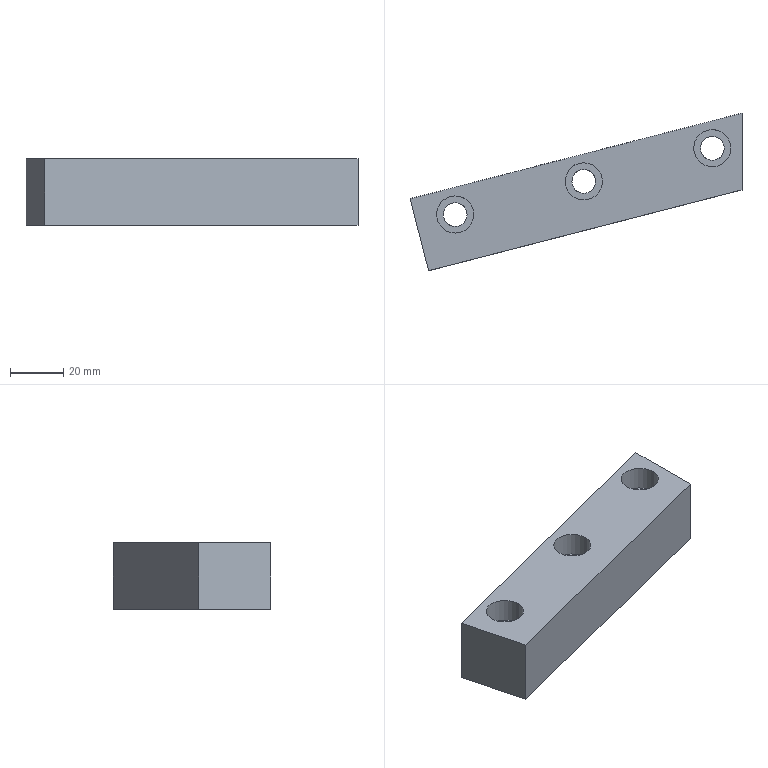Part | STEP file | 车灯-后视镜_id58_x_t | 1 solid | 15 faces | box 125 x 59.346 x 25 mm | volume 80625 mm3 | plane 9 | cylinder 6 | commonest cylinder face diameters 9 x3 14 x3
STEP:
#1=CARTESIAN_POINT('',(-243.008,55.534,-0.2856));
#2=VERTEX_POINT('',#1);
#3=CARTESIAN_POINT('',(-250.,82.647,-0.2856));
#4=VERTEX_POINT('',#3);
#5=CARTESIAN_POINT('',(-243.008,55.534,-0.2856));
#6=DIRECTION('',(-0.2497,0.9683,0.));
#7=VECTOR('',#6,1.);
#8=LINE('',#5,#7);
#9=EDGE_CURVE('',#2,#4,#8,.T.);
#10=ORIENTED_EDGE('',*,*,#9,.T.);
#11=CARTESIAN_POINT('',(-250.,82.647,-25.286));
#12=VERTEX_POINT('',#11);
#13=CARTESIAN_POINT('',(-250.,82.647,-25.286));
#14=DIRECTION('',(0.,0.,-1.));
#15=VECTOR('',#14,1.);
#16=LINE('',#13,#15);
#17=EDGE_CURVE('',#4,#12,#16,.T.);
#18=ORIENTED_EDGE('',*,*,#17,.T.);
#19=CARTESIAN_POINT('',(-243.008,55.534,-25.286));
#20=VERTEX_POINT('',#19);
#21=CARTESIAN_POINT('',(-243.008,55.534,-25.286));
#22=DIRECTION('',(0.2497,-0.9683,0.));
#23=VECTOR('',#22,1.);
#24=LINE('',#21,#23);
#25=EDGE_CURVE('',#12,#20,#24,.T.);
#26=ORIENTED_EDGE('',*,*,#25,.T.);
#27=CARTESIAN_POINT('',(-243.008,55.534,-25.286));
#28=DIRECTION('',(0.,0.,-1.));
#29=VECTOR('',#28,1.);
#30=LINE('',#27,#29);
#31=EDGE_CURVE('',#2,#20,#30,.T.);
#32=ORIENTED_EDGE('',*,*,#31,.F.);
#33=EDGE_LOOP('',(#10,#18,#26,#32));
#34=FACE_OUTER_BOUND('',#33,.T.);
#35=CARTESIAN_POINT('',(-250.,82.647,-0.5));
#36=DIRECTION('',(-0.9683,-0.2497,0.));
#37=DIRECTION('',(0.2497,-0.9683,0.));
#38=AXIS2_PLACEMENT_3D('',#35,#36,#37);
#39=PLANE('',#38);
#40=ADVANCED_FACE('',(#34),#39,.T.);
#41=CARTESIAN_POINT('',(-125.,85.965,-0.2856));
#42=VERTEX_POINT('',#41);
#43=CARTESIAN_POINT('',(-125.,114.881,-0.2856));
#44=VERTEX_POINT('',#43);
#45=CARTESIAN_POINT('',(-125.,90.74,-0.2856));
#46=DIRECTION('',(0.,1.,0.));
#47=VECTOR('',#46,1.);
#48=LINE('',#45,#47);
#49=EDGE_CURVE('',#42,#44,#48,.T.);
#50=ORIENTED_EDGE('',*,*,#49,.F.);
#51=CARTESIAN_POINT('',(-125.,85.965,-25.286));
#52=VERTEX_POINT('',#51);
#53=CARTESIAN_POINT('',(-125.,85.965,-25.286));
#54=DIRECTION('',(0.,0.,-1.));
#55=VECTOR('',#54,1.);
#56=LINE('',#53,#55);
#57=EDGE_CURVE('',#42,#52,#56,.T.);
#58=ORIENTED_EDGE('',*,*,#57,.T.);
#59=CARTESIAN_POINT('',(-125.,114.881,-25.286));
#60=VERTEX_POINT('',#59);
#61=CARTESIAN_POINT('',(-125.,90.74,-25.286));
#62=DIRECTION('',(0.,-1.,0.));
#63=VECTOR('',#62,1.);
#64=LINE('',#61,#63);
#65=EDGE_CURVE('',#60,#52,#64,.T.);
#66=ORIENTED_EDGE('',*,*,#65,.F.);
#67=CARTESIAN_POINT('',(-125.,114.881,-25.286));
#68=DIRECTION('',(0.,0.,-1.));
#69=VECTOR('',#68,1.);
#70=LINE('',#67,#69);
#71=EDGE_CURVE('',#44,#60,#70,.T.);
#72=ORIENTED_EDGE('',*,*,#71,.F.);
#73=EDGE_LOOP('',(#50,#58,#66,#72));
#74=FACE_OUTER_BOUND('',#73,.T.);
#75=CARTESIAN_POINT('',(-125.,85.965,-35.286));
#76=DIRECTION('',(-1.,0.,0.));
#77=DIRECTION('',(0.,0.,1.));
#78=AXIS2_PLACEMENT_3D('',#75,#76,#77);
#79=PLANE('',#78);
#80=ADVANCED_FACE('',(#74),#79,.F.);
#81=ORIENTED_EDGE('',*,*,#17,.F.);
#82=CARTESIAN_POINT('',(-113.474,117.853,-0.2856));
#83=DIRECTION('',(-0.9683,-0.2497,0.));
#84=VECTOR('',#83,1.);
#85=LINE('',#82,#84);
#86=EDGE_CURVE('',#44,#4,#85,.T.);
#87=ORIENTED_EDGE('',*,*,#86,.F.);
#88=ORIENTED_EDGE('',*,*,#71,.T.);
#89=CARTESIAN_POINT('',(-113.474,117.853,-25.286));
#90=DIRECTION('',(-0.9683,-0.2497,0.));
#91=VECTOR('',#90,1.);
#92=LINE('',#89,#91);
#93=EDGE_CURVE('',#60,#12,#92,.T.);
#94=ORIENTED_EDGE('',*,*,#93,.T.);
#95=EDGE_LOOP('',(#81,#87,#88,#94));
#96=FACE_OUTER_BOUND('',#95,.T.);
#97=CARTESIAN_POINT('',(-113.474,117.853,-25.286));
#98=DIRECTION('',(0.2497,-0.9683,0.));
#99=DIRECTION('',(-0.9683,-0.2497,0.));
#100=AXIS2_PLACEMENT_3D('',#97,#98,#99);
#101=PLANE('',#100);
#102=ADVANCED_FACE('',(#96),#101,.F.);
#103=CARTESIAN_POINT('',(-106.483,90.74,-0.2856));
#104=DIRECTION('',(-0.9683,-0.2497,0.));
#105=VECTOR('',#104,1.);
#106=LINE('',#103,#105);
#107=EDGE_CURVE('',#42,#2,#106,.T.);
#108=ORIENTED_EDGE('',*,*,#107,.T.);
#109=ORIENTED_EDGE('',*,*,#31,.T.);
#110=CARTESIAN_POINT('',(-106.483,90.74,-25.286));
#111=DIRECTION('',(-0.9683,-0.2497,0.));
#112=VECTOR('',#111,1.);
#113=LINE('',#110,#112);
#114=EDGE_CURVE('',#52,#20,#113,.T.);
#115=ORIENTED_EDGE('',*,*,#114,.F.);
#116=ORIENTED_EDGE('',*,*,#57,.F.);
#117=EDGE_LOOP('',(#108,#109,#115,#116));
#118=FACE_OUTER_BOUND('',#117,.T.);
#119=CARTESIAN_POINT('',(-106.483,90.74,-25.286));
#120=DIRECTION('',(0.2497,-0.9683,0.));
#121=DIRECTION('',(-0.9683,-0.2497,0.));
#122=AXIS2_PLACEMENT_3D('',#119,#120,#121);
#123=PLANE('',#122);
#124=ADVANCED_FACE('',(#118),#123,.T.);
#125=CARTESIAN_POINT('',(-134.406,94.899,-0.2856));
#126=VERTEX_POINT('',#125);
#127=CARTESIAN_POINT('',(-136.154,101.677,-0.2856));
#128=DIRECTION('',(0.,0.,-1.));
#129=DIRECTION('',(0.2497,-0.9683,0.));
#130=AXIS2_PLACEMENT_3D('',#127,#128,#129);
#131=CIRCLE('',#130,7.);
#132=EDGE_CURVE('',#126,#126,#131,.T.);
#133=ORIENTED_EDGE('',*,*,#132,.T.);
#134=EDGE_LOOP('',(#133));
#135=FACE_BOUND('',#134,.T.);
#136=CARTESIAN_POINT('',(-182.822,82.414,-0.2856));
#137=VERTEX_POINT('',#136);
#138=CARTESIAN_POINT('',(-184.57,89.192,-0.2856));
#139=DIRECTION('',(0.,0.,-1.));
#140=DIRECTION('',(0.2497,-0.9683,0.));
#141=AXIS2_PLACEMENT_3D('',#138,#139,#140);
#142=CIRCLE('',#141,7.);
#143=EDGE_CURVE('',#137,#137,#142,.T.);
#144=ORIENTED_EDGE('',*,*,#143,.T.);
#145=EDGE_LOOP('',(#144));
#146=FACE_BOUND('',#145,.T.);
#147=CARTESIAN_POINT('',(-231.238,69.929,-0.2856));
#148=VERTEX_POINT('',#147);
#149=CARTESIAN_POINT('',(-232.986,76.707,-0.2856));
#150=DIRECTION('',(0.,0.,-1.));
#151=DIRECTION('',(0.2497,-0.9683,0.));
#152=AXIS2_PLACEMENT_3D('',#149,#150,#151);
#153=CIRCLE('',#152,7.);
#154=EDGE_CURVE('',#148,#148,#153,.T.);
#155=ORIENTED_EDGE('',*,*,#154,.T.);
#156=EDGE_LOOP('',(#155));
#157=FACE_BOUND('',#156,.T.);
#158=ORIENTED_EDGE('',*,*,#9,.F.);
#159=ORIENTED_EDGE('',*,*,#107,.F.);
#160=ORIENTED_EDGE('',*,*,#49,.T.);
#161=ORIENTED_EDGE('',*,*,#86,.T.);
#162=EDGE_LOOP('',(#158,#159,#160,#161));
#163=FACE_BOUND('',#162,.T.);
#164=CARTESIAN_POINT('',(-106.483,90.74,-0.2856));
#165=DIRECTION('',(0.,0.,-1.));
#166=DIRECTION('',(-0.9683,-0.2497,0.));
#167=AXIS2_PLACEMENT_3D('',#164,#165,#166);
#168=PLANE('',#167);
#169=ADVANCED_FACE('',(#135,#146,#157,#163),#168,.F.);
#170=CARTESIAN_POINT('',(-135.03,97.32,-25.286));
#171=VERTEX_POINT('',#170);
#172=CARTESIAN_POINT('',(-136.154,101.677,-25.286));
#173=DIRECTION('',(0.,0.,1.));
#174=DIRECTION('',(0.2497,-0.9683,0.));
#175=AXIS2_PLACEMENT_3D('',#172,#173,#174);
#176=CIRCLE('',#175,4.5);
#177=EDGE_CURVE('',#171,#171,#176,.T.);
#178=ORIENTED_EDGE('',*,*,#177,.T.);
#179=EDGE_LOOP('',(#178));
#180=FACE_BOUND('',#179,.T.);
#181=CARTESIAN_POINT('',(-183.446,84.835,-25.286));
#182=VERTEX_POINT('',#181);
#183=CARTESIAN_POINT('',(-184.57,89.192,-25.286));
#184=DIRECTION('',(0.,0.,1.));
#185=DIRECTION('',(0.2497,-0.9683,0.));
#186=AXIS2_PLACEMENT_3D('',#183,#184,#185);
#187=CIRCLE('',#186,4.5);
#188=EDGE_CURVE('',#182,#182,#187,.T.);
#189=ORIENTED_EDGE('',*,*,#188,.T.);
#190=EDGE_LOOP('',(#189));
#191=FACE_BOUND('',#190,.T.);
#192=CARTESIAN_POINT('',(-231.863,72.35,-25.286));
#193=VERTEX_POINT('',#192);
#194=CARTESIAN_POINT('',(-232.986,76.707,-25.286));
#195=DIRECTION('',(0.,0.,1.));
#196=DIRECTION('',(0.2497,-0.9683,0.));
#197=AXIS2_PLACEMENT_3D('',#194,#195,#196);
#198=CIRCLE('',#197,4.5);
#199=EDGE_CURVE('',#193,#193,#198,.T.);
#200=ORIENTED_EDGE('',*,*,#199,.T.);
#201=EDGE_LOOP('',(#200));
#202=FACE_BOUND('',#201,.T.);
#203=ORIENTED_EDGE('',*,*,#25,.F.);
#204=ORIENTED_EDGE('',*,*,#93,.F.);
#205=ORIENTED_EDGE('',*,*,#65,.T.);
#206=ORIENTED_EDGE('',*,*,#114,.T.);
#207=EDGE_LOOP('',(#203,#204,#205,#206));
#208=FACE_BOUND('',#207,.T.);
#209=CARTESIAN_POINT('',(-106.483,90.74,-25.286));
#210=DIRECTION('',(0.,0.,-1.));
#211=DIRECTION('',(-0.9683,-0.2497,0.));
#212=AXIS2_PLACEMENT_3D('',#209,#210,#211);
#213=PLANE('',#212);
#214=ADVANCED_FACE('',(#180,#191,#202,#208),#213,.T.);
#215=CARTESIAN_POINT('',(-237.486,76.707,-9.286));
#216=VERTEX_POINT('',#215);
#217=CARTESIAN_POINT('',(-232.986,76.707,-9.286));
#218=DIRECTION('',(0.,0.,1.));
#219=DIRECTION('',(-1.,0.,0.));
#220=AXIS2_PLACEMENT_3D('',#217,#218,#219);
#221=CIRCLE('',#220,4.5);
#222=EDGE_CURVE('',#216,#216,#221,.T.);
#223=ORIENTED_EDGE('',*,*,#222,.T.);
#224=EDGE_LOOP('',(#223));
#225=FACE_BOUND('',#224,.T.);
#226=ORIENTED_EDGE('',*,*,#199,.F.);
#227=EDGE_LOOP('',(#226));
#228=FACE_BOUND('',#227,.T.);
#229=CARTESIAN_POINT('',(-232.986,76.707,-24.786));
#230=DIRECTION('',(0.,0.,1.));
#231=DIRECTION('',(-0.2497,0.9683,0.));
#232=AXIS2_PLACEMENT_3D('',#229,#230,#231);
#233=CYLINDRICAL_SURFACE('',#232,4.5);
#234=ADVANCED_FACE('',(#225,#228),#233,.F.);
#235=ORIENTED_EDGE('',*,*,#222,.F.);
#236=EDGE_LOOP('',(#235));
#237=FACE_BOUND('',#236,.T.);
#238=CARTESIAN_POINT('',(-234.734,83.486,-9.286));
#239=VERTEX_POINT('',#238);
#240=CARTESIAN_POINT('',(-232.986,76.707,-9.286));
#241=DIRECTION('',(0.,0.,1.));
#242=DIRECTION('',(-0.2497,0.9683,0.));
#243=AXIS2_PLACEMENT_3D('',#240,#241,#242);
#244=CIRCLE('',#243,7.);
#245=EDGE_CURVE('',#239,#239,#244,.T.);
#246=ORIENTED_EDGE('',*,*,#245,.T.);
#247=EDGE_LOOP('',(#246));
#248=FACE_BOUND('',#247,.T.);
#249=CARTESIAN_POINT('',(-232.986,76.707,-9.286));
#250=DIRECTION('',(0.,0.,-1.));
#251=DIRECTION('',(0.2497,-0.9683,0.));
#252=AXIS2_PLACEMENT_3D('',#249,#250,#251);
#253=PLANE('',#252);
#254=ADVANCED_FACE('',(#237,#248),#253,.F.);
#255=ORIENTED_EDGE('',*,*,#245,.F.);
#256=EDGE_LOOP('',(#255));
#257=FACE_BOUND('',#256,.T.);
#258=ORIENTED_EDGE('',*,*,#154,.F.);
#259=EDGE_LOOP('',(#258));
#260=FACE_BOUND('',#259,.T.);
#261=CARTESIAN_POINT('',(-232.986,76.707,-0.2856));
#262=DIRECTION('',(0.,0.,-1.));
#263=DIRECTION('',(0.2497,-0.9683,0.));
#264=AXIS2_PLACEMENT_3D('',#261,#262,#263);
#265=CYLINDRICAL_SURFACE('',#264,7.);
#266=ADVANCED_FACE('',(#257,#260),#265,.F.);
#267=CARTESIAN_POINT('',(-189.07,89.192,-9.286));
#268=VERTEX_POINT('',#267);
#269=CARTESIAN_POINT('',(-184.57,89.192,-9.286));
#270=DIRECTION('',(0.,0.,1.));
#271=DIRECTION('',(-1.,0.,0.));
#272=AXIS2_PLACEMENT_3D('',#269,#270,#271);
#273=CIRCLE('',#272,4.5);
#274=EDGE_CURVE('',#268,#268,#273,.T.);
#275=ORIENTED_EDGE('',*,*,#274,.T.);
#276=EDGE_LOOP('',(#275));
#277=FACE_BOUND('',#276,.T.);
#278=ORIENTED_EDGE('',*,*,#188,.F.);
#279=EDGE_LOOP('',(#278));
#280=FACE_BOUND('',#279,.T.);
#281=CARTESIAN_POINT('',(-184.57,89.192,-24.786));
#282=DIRECTION('',(0.,0.,1.));
#283=DIRECTION('',(-0.2497,0.9683,0.));
#284=AXIS2_PLACEMENT_3D('',#281,#282,#283);
#285=CYLINDRICAL_SURFACE('',#284,4.5);
#286=ADVANCED_FACE('',(#277,#280),#285,.F.);
#287=ORIENTED_EDGE('',*,*,#274,.F.);
#288=EDGE_LOOP('',(#287));
#289=FACE_BOUND('',#288,.T.);
#290=CARTESIAN_POINT('',(-186.318,95.971,-9.286));
#291=VERTEX_POINT('',#290);
#292=CARTESIAN_POINT('',(-184.57,89.192,-9.286));
#293=DIRECTION('',(0.,0.,1.));
#294=DIRECTION('',(-0.2497,0.9683,0.));
#295=AXIS2_PLACEMENT_3D('',#292,#293,#294);
#296=CIRCLE('',#295,7.);
#297=EDGE_CURVE('',#291,#291,#296,.T.);
#298=ORIENTED_EDGE('',*,*,#297,.T.);
#299=EDGE_LOOP('',(#298));
#300=FACE_BOUND('',#299,.T.);
#301=CARTESIAN_POINT('',(-184.57,89.192,-9.286));
#302=DIRECTION('',(0.,0.,-1.));
#303=DIRECTION('',(0.2497,-0.9683,0.));
#304=AXIS2_PLACEMENT_3D('',#301,#302,#303);
#305=PLANE('',#304);
#306=ADVANCED_FACE('',(#289,#300),#305,.F.);
#307=ORIENTED_EDGE('',*,*,#297,.F.);
#308=EDGE_LOOP('',(#307));
#309=FACE_BOUND('',#308,.T.);
#310=ORIENTED_EDGE('',*,*,#143,.F.);
#311=EDGE_LOOP('',(#310));
#312=FACE_BOUND('',#311,.T.);
#313=CARTESIAN_POINT('',(-184.57,89.192,-0.2856));
#314=DIRECTION('',(0.,0.,-1.));
#315=DIRECTION('',(0.2497,-0.9683,0.));
#316=AXIS2_PLACEMENT_3D('',#313,#314,#315);
#317=CYLINDRICAL_SURFACE('',#316,7.);
#318=ADVANCED_FACE('',(#309,#312),#317,.F.);
#319=CARTESIAN_POINT('',(-140.654,101.677,-9.286));
#320=VERTEX_POINT('',#319);
#321=CARTESIAN_POINT('',(-136.154,101.677,-9.286));
#322=DIRECTION('',(0.,0.,1.));
#323=DIRECTION('',(-1.,0.,0.));
#324=AXIS2_PLACEMENT_3D('',#321,#322,#323);
#325=CIRCLE('',#324,4.5);
#326=EDGE_CURVE('',#320,#320,#325,.T.);
#327=ORIENTED_EDGE('',*,*,#326,.T.);
#328=EDGE_LOOP('',(#327));
#329=FACE_BOUND('',#328,.T.);
#330=ORIENTED_EDGE('',*,*,#177,.F.);
#331=EDGE_LOOP('',(#330));
#332=FACE_BOUND('',#331,.T.);
#333=CARTESIAN_POINT('',(-136.154,101.677,-24.786));
#334=DIRECTION('',(0.,0.,1.));
#335=DIRECTION('',(-0.2497,0.9683,0.));
#336=AXIS2_PLACEMENT_3D('',#333,#334,#335);
#337=CYLINDRICAL_SURFACE('',#336,4.5);
#338=ADVANCED_FACE('',(#329,#332),#337,.F.);
#339=ORIENTED_EDGE('',*,*,#326,.F.);
#340=EDGE_LOOP('',(#339));
#341=FACE_BOUND('',#340,.T.);
#342=CARTESIAN_POINT('',(-137.902,108.455,-9.286));
#343=VERTEX_POINT('',#342);
#344=CARTESIAN_POINT('',(-136.154,101.677,-9.286));
#345=DIRECTION('',(0.,0.,1.));
#346=DIRECTION('',(-0.2497,0.9683,0.));
#347=AXIS2_PLACEMENT_3D('',#344,#345,#346);
#348=CIRCLE('',#347,7.);
#349=EDGE_CURVE('',#343,#343,#348,.T.);
#350=ORIENTED_EDGE('',*,*,#349,.T.);
#351=EDGE_LOOP('',(#350));
#352=FACE_BOUND('',#351,.T.);
#353=CARTESIAN_POINT('',(-136.154,101.677,-9.286));
#354=DIRECTION('',(0.,0.,-1.));
#355=DIRECTION('',(0.2497,-0.9683,0.));
#356=AXIS2_PLACEMENT_3D('',#353,#354,#355);
#357=PLANE('',#356);
#358=ADVANCED_FACE('',(#341,#352),#357,.F.);
#359=ORIENTED_EDGE('',*,*,#349,.F.);
#360=EDGE_LOOP('',(#359));
#361=FACE_BOUND('',#360,.T.);
#362=ORIENTED_EDGE('',*,*,#132,.F.);
#363=EDGE_LOOP('',(#362));
#364=FACE_BOUND('',#363,.T.);
#365=CARTESIAN_POINT('',(-136.154,101.677,-0.2856));
#366=DIRECTION('',(0.,0.,-1.));
#367=DIRECTION('',(0.2497,-0.9683,0.));
#368=AXIS2_PLACEMENT_3D('',#365,#366,#367);
#369=CYLINDRICAL_SURFACE('',#368,7.);
#370=ADVANCED_FACE('',(#361,#364),#369,.F.);
#371=CLOSED_SHELL('',(#40,#80,#102,#124,#169,#214,#234,#254,#266,#286,#306,#318,#338,#358,#370));
#372=MANIFOLD_SOLID_BREP('',#371);
#373=(LENGTH_UNIT()NAMED_UNIT(*)SI_UNIT(.MILLI.,.METRE.));
#374=UNCERTAINTY_MEASURE_WITH_UNIT(LENGTH_MEASURE(0.00002),#373,'','');
#375=(NAMED_UNIT(*)PLANE_ANGLE_UNIT()SI_UNIT($,.RADIAN.));
#376=PLANE_ANGLE_MEASURE_WITH_UNIT(PLANE_ANGLE_MEASURE(0.01745),#375);
#377=DIMENSIONAL_EXPONENTS(0.,0.,0.,0.,0.,0.,0.);
#378=(CONVERSION_BASED_UNIT('DEGREE',#376)NAMED_UNIT(#377)PLANE_ANGLE_UNIT());
#379=(NAMED_UNIT(*)SI_UNIT($,.STERADIAN.)SOLID_ANGLE_UNIT());
#380=(GEOMETRIC_REPRESENTATION_CONTEXT(3)GLOBAL_UNCERTAINTY_ASSIGNED_CONTEXT((#374))GLOBAL_UNIT_ASSIGNED_CONTEXT((#373,#378,#379))REPRESENTATION_CONTEXT('',''));
#381=ADVANCED_BREP_SHAPE_REPRESENTATION('',(#372),#380);